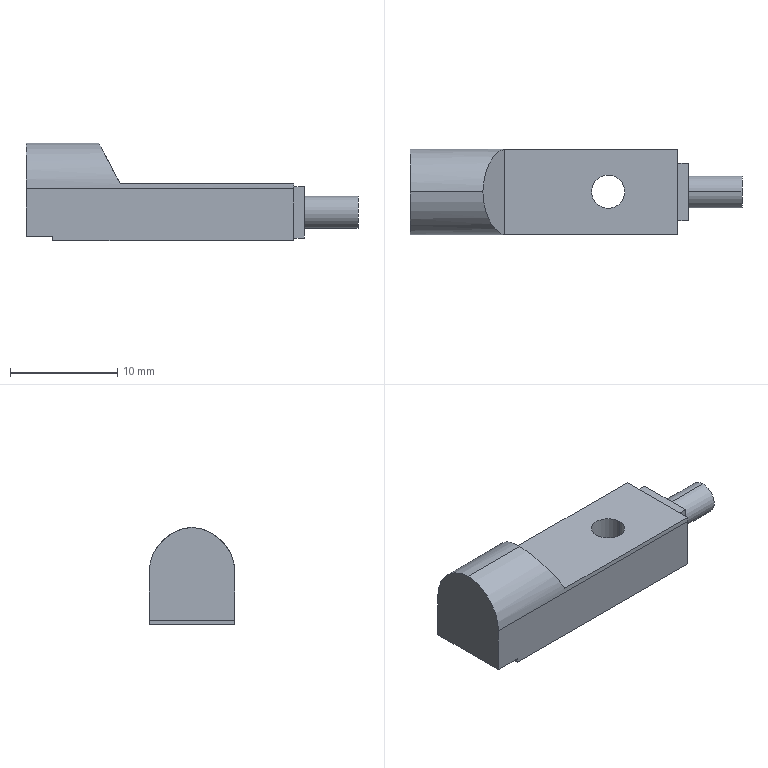Part | SolidWorks | features ICE 4, Extrusion 1, Fillet 1 | 1 solid | 21 faces | box 31 x 8 x 9.093 mm | volume 1254 mm3 | plane 15 | cylinder 6 | commonest cylinder face diameters 3 x2 3.1 x2 8.5 x2
STEP:
#1=CARTESIAN_POINT('',(31.,4.,1.15));
#2=VERTEX_POINT('',#1);
#3=CARTESIAN_POINT('',(31.,4.,4.15));
#4=VERTEX_POINT('',#3);
#5=CARTESIAN_POINT('',(31.,4.,2.65));
#6=DIRECTION('',(1.,0.,0.));
#7=DIRECTION('',(0.,0.,-1.));
#8=AXIS2_PLACEMENT_3D('',#5,#6,#7);
#9=CIRCLE('',#8,1.5);
#10=EDGE_CURVE('',#2,#4,#9,.T.);
#11=ORIENTED_EDGE('',*,*,#10,.F.);
#12=CARTESIAN_POINT('',(26.,4.,1.15));
#13=VERTEX_POINT('',#12);
#14=CARTESIAN_POINT('',(31.,4.,1.15));
#15=DIRECTION('',(-1.,0.,0.));
#16=VECTOR('',#15,1000.);
#17=LINE('',#14,#16);
#18=EDGE_CURVE('',#2,#13,#17,.T.);
#19=ORIENTED_EDGE('',*,*,#18,.T.);
#20=CARTESIAN_POINT('',(26.,4.,4.15));
#21=VERTEX_POINT('',#20);
#22=CARTESIAN_POINT('',(26.,4.,2.65));
#23=DIRECTION('',(1.,0.,0.));
#24=DIRECTION('',(0.,0.,-1.));
#25=AXIS2_PLACEMENT_3D('',#22,#23,#24);
#26=CIRCLE('',#25,1.5);
#27=EDGE_CURVE('',#13,#21,#26,.T.);
#28=ORIENTED_EDGE('',*,*,#27,.T.);
#29=CARTESIAN_POINT('',(31.,4.,4.15));
#30=DIRECTION('',(-1.,0.,0.));
#31=VECTOR('',#30,1000.);
#32=LINE('',#29,#31);
#33=EDGE_CURVE('',#4,#21,#32,.T.);
#34=ORIENTED_EDGE('',*,*,#33,.F.);
#35=EDGE_LOOP('',(#11,#19,#28,#34));
#36=FACE_OUTER_BOUND('',#35,.T.);
#37=CARTESIAN_POINT('',(31.,4.,2.65));
#38=DIRECTION('',(-1.,0.,0.));
#39=DIRECTION('',(0.,0.,1.));
#40=AXIS2_PLACEMENT_3D('',#37,#38,#39);
#41=CYLINDRICAL_SURFACE('',#40,1.5);
#42=ADVANCED_FACE('',(#36),#41,.T.);
#43=CARTESIAN_POINT('',(20.05,4.024,0.));
#44=VERTEX_POINT('',#43);
#45=CARTESIAN_POINT('',(16.95,4.024,0.));
#46=VERTEX_POINT('',#45);
#47=CARTESIAN_POINT('',(18.5,4.024,0.));
#48=DIRECTION('',(0.,0.,-1.));
#49=DIRECTION('',(-1.,0.,0.));
#50=AXIS2_PLACEMENT_3D('',#47,#48,#49);
#51=CIRCLE('',#50,1.55);
#52=EDGE_CURVE('',#44,#46,#51,.T.);
#53=ORIENTED_EDGE('',*,*,#52,.T.);
#54=CARTESIAN_POINT('',(16.95,4.024,5.3));
#55=VERTEX_POINT('',#54);
#56=CARTESIAN_POINT('',(16.95,4.024,-2.9));
#57=DIRECTION('',(0.,0.,1.));
#58=VECTOR('',#57,1000.);
#59=LINE('',#56,#58);
#60=EDGE_CURVE('',#46,#55,#59,.T.);
#61=ORIENTED_EDGE('',*,*,#60,.T.);
#62=CARTESIAN_POINT('',(20.05,4.024,5.3));
#63=VERTEX_POINT('',#62);
#64=CARTESIAN_POINT('',(18.5,4.024,5.3));
#65=DIRECTION('',(0.,0.,1.));
#66=DIRECTION('',(1.,0.,0.));
#67=AXIS2_PLACEMENT_3D('',#64,#65,#66);
#68=CIRCLE('',#67,1.55);
#69=EDGE_CURVE('',#55,#63,#68,.T.);
#70=ORIENTED_EDGE('',*,*,#69,.T.);
#71=CARTESIAN_POINT('',(20.05,4.024,-2.9));
#72=DIRECTION('',(0.,0.,1.));
#73=VECTOR('',#72,1000.);
#74=LINE('',#71,#73);
#75=EDGE_CURVE('',#44,#63,#74,.T.);
#76=ORIENTED_EDGE('',*,*,#75,.F.);
#77=EDGE_LOOP('',(#53,#61,#70,#76));
#78=FACE_OUTER_BOUND('',#77,.T.);
#79=CARTESIAN_POINT('',(18.5,4.024,-2.9));
#80=DIRECTION('',(0.,0.,1.));
#81=DIRECTION('',(1.,0.,0.));
#82=AXIS2_PLACEMENT_3D('',#79,#80,#81);
#83=CYLINDRICAL_SURFACE('',#82,1.55);
#84=ADVANCED_FACE('',(#78),#83,.F.);
#85=CARTESIAN_POINT('',(26.,1.3,0.25));
#86=VERTEX_POINT('',#85);
#87=CARTESIAN_POINT('',(26.,6.7,0.25));
#88=VERTEX_POINT('',#87);
#89=CARTESIAN_POINT('',(26.,6.7,0.25));
#90=DIRECTION('',(0.,1.,0.));
#91=VECTOR('',#90,1000.);
#92=LINE('',#89,#91);
#93=EDGE_CURVE('',#86,#88,#92,.T.);
#94=ORIENTED_EDGE('',*,*,#93,.T.);
#95=CARTESIAN_POINT('',(26.,6.7,5.05));
#96=VERTEX_POINT('',#95);
#97=CARTESIAN_POINT('',(26.,6.7,5.05));
#98=DIRECTION('',(0.,0.,1.));
#99=VECTOR('',#98,1000.);
#100=LINE('',#97,#99);
#101=EDGE_CURVE('',#88,#96,#100,.T.);
#102=ORIENTED_EDGE('',*,*,#101,.T.);
#103=CARTESIAN_POINT('',(26.,1.3,5.05));
#104=VERTEX_POINT('',#103);
#105=CARTESIAN_POINT('',(26.,6.7,5.05));
#106=DIRECTION('',(0.,-1.,0.));
#107=VECTOR('',#106,1000.);
#108=LINE('',#105,#107);
#109=EDGE_CURVE('',#96,#104,#108,.T.);
#110=ORIENTED_EDGE('',*,*,#109,.T.);
#111=CARTESIAN_POINT('',(26.,1.3,5.05));
#112=DIRECTION('',(0.,0.,-1.));
#113=VECTOR('',#112,1000.);
#114=LINE('',#111,#113);
#115=EDGE_CURVE('',#104,#86,#114,.T.);
#116=ORIENTED_EDGE('',*,*,#115,.T.);
#117=EDGE_LOOP('',(#94,#102,#110,#116));
#118=FACE_OUTER_BOUND('',#117,.T.);
#119=CARTESIAN_POINT('',(26.,4.,2.65));
#120=DIRECTION('',(1.,0.,0.));
#121=DIRECTION('',(0.,0.,-1.));
#122=AXIS2_PLACEMENT_3D('',#119,#120,#121);
#123=CIRCLE('',#122,1.5);
#124=EDGE_CURVE('',#21,#13,#123,.T.);
#125=ORIENTED_EDGE('',*,*,#124,.F.);
#126=ORIENTED_EDGE('',*,*,#27,.F.);
#127=EDGE_LOOP('',(#125,#126));
#128=FACE_BOUND('',#127,.T.);
#129=CARTESIAN_POINT('',(26.,1.3,0.25));
#130=DIRECTION('',(1.,0.,0.));
#131=DIRECTION('',(0.,0.,-1.));
#132=AXIS2_PLACEMENT_3D('',#129,#130,#131);
#133=PLANE('',#132);
#134=ADVANCED_FACE('',(#118,#128),#133,.T.);
#135=CARTESIAN_POINT('',(25.,8.,4.85));
#136=VERTEX_POINT('',#135);
#137=CARTESIAN_POINT('',(25.,8.,0.));
#138=VERTEX_POINT('',#137);
#139=CARTESIAN_POINT('',(25.,8.,9.1));
#140=DIRECTION('',(0.,0.,-1.));
#141=VECTOR('',#140,1000.);
#142=LINE('',#139,#141);
#143=EDGE_CURVE('',#136,#138,#142,.T.);
#144=ORIENTED_EDGE('',*,*,#143,.F.);
#145=CARTESIAN_POINT('',(25.,7.976,5.3));
#146=VERTEX_POINT('',#145);
#147=CARTESIAN_POINT('',(25.,3.75,4.85));
#148=DIRECTION('',(1.,0.,0.));
#149=DIRECTION('',(0.,0.,1.));
#150=AXIS2_PLACEMENT_3D('',#147,#148,#149);
#151=CIRCLE('',#150,4.25);
#152=EDGE_CURVE('',#136,#146,#151,.T.);
#153=ORIENTED_EDGE('',*,*,#152,.T.);
#154=CARTESIAN_POINT('',(25.,0.02389,5.3));
#155=VERTEX_POINT('',#154);
#156=CARTESIAN_POINT('',(25.,8.2,5.3));
#157=DIRECTION('',(0.,-1.,0.));
#158=VECTOR('',#157,1000.);
#159=LINE('',#156,#158);
#160=EDGE_CURVE('',#146,#155,#159,.T.);
#161=ORIENTED_EDGE('',*,*,#160,.T.);
#162=CARTESIAN_POINT('',(25.,0.,4.85));
#163=VERTEX_POINT('',#162);
#164=CARTESIAN_POINT('',(25.,4.25,4.85));
#165=DIRECTION('',(1.,0.,0.));
#166=DIRECTION('',(0.,0.,1.));
#167=AXIS2_PLACEMENT_3D('',#164,#165,#166);
#168=CIRCLE('',#167,4.25);
#169=EDGE_CURVE('',#155,#163,#168,.T.);
#170=ORIENTED_EDGE('',*,*,#169,.T.);
#171=CARTESIAN_POINT('',(25.,0.,0.));
#172=VERTEX_POINT('',#171);
#173=CARTESIAN_POINT('',(25.,0.,9.1));
#174=DIRECTION('',(0.,0.,-1.));
#175=VECTOR('',#174,1000.);
#176=LINE('',#173,#175);
#177=EDGE_CURVE('',#163,#172,#176,.T.);
#178=ORIENTED_EDGE('',*,*,#177,.T.);
#179=CARTESIAN_POINT('',(25.,0.,0.));
#180=DIRECTION('',(0.,1.,0.));
#181=VECTOR('',#180,1000.);
#182=LINE('',#179,#181);
#183=EDGE_CURVE('',#172,#138,#182,.T.);
#184=ORIENTED_EDGE('',*,*,#183,.T.);
#185=EDGE_LOOP('',(#144,#153,#161,#170,#178,#184));
#186=FACE_OUTER_BOUND('',#185,.T.);
#187=CARTESIAN_POINT('',(25.,1.3,0.25));
#188=VERTEX_POINT('',#187);
#189=CARTESIAN_POINT('',(25.,6.7,0.25));
#190=VERTEX_POINT('',#189);
#191=CARTESIAN_POINT('',(25.,6.7,0.25));
#192=DIRECTION('',(0.,1.,0.));
#193=VECTOR('',#192,1000.);
#194=LINE('',#191,#193);
#195=EDGE_CURVE('',#188,#190,#194,.T.);
#196=ORIENTED_EDGE('',*,*,#195,.F.);
#197=CARTESIAN_POINT('',(25.,1.3,5.05));
#198=VERTEX_POINT('',#197);
#199=CARTESIAN_POINT('',(25.,1.3,5.05));
#200=DIRECTION('',(0.,0.,-1.));
#201=VECTOR('',#200,1000.);
#202=LINE('',#199,#201);
#203=EDGE_CURVE('',#198,#188,#202,.T.);
#204=ORIENTED_EDGE('',*,*,#203,.F.);
#205=CARTESIAN_POINT('',(25.,6.7,5.05));
#206=VERTEX_POINT('',#205);
#207=CARTESIAN_POINT('',(25.,6.7,5.05));
#208=DIRECTION('',(0.,-1.,0.));
#209=VECTOR('',#208,1000.);
#210=LINE('',#207,#209);
#211=EDGE_CURVE('',#206,#198,#210,.T.);
#212=ORIENTED_EDGE('',*,*,#211,.F.);
#213=CARTESIAN_POINT('',(25.,6.7,5.05));
#214=DIRECTION('',(0.,0.,1.));
#215=VECTOR('',#214,1000.);
#216=LINE('',#213,#215);
#217=EDGE_CURVE('',#190,#206,#216,.T.);
#218=ORIENTED_EDGE('',*,*,#217,.F.);
#219=EDGE_LOOP('',(#196,#204,#212,#218));
#220=FACE_BOUND('',#219,.T.);
#221=CARTESIAN_POINT('',(25.,0.,9.1));
#222=DIRECTION('',(-1.,0.,0.));
#223=DIRECTION('',(0.,0.,1.));
#224=AXIS2_PLACEMENT_3D('',#221,#222,#223);
#225=PLANE('',#224);
#226=ADVANCED_FACE('',(#186,#220),#225,.F.);
#227=CARTESIAN_POINT('',(0.,0.,4.85));
#228=VERTEX_POINT('',#227);
#229=CARTESIAN_POINT('',(0.,4.,9.093));
#230=VERTEX_POINT('',#229);
#231=CARTESIAN_POINT('',(0.,4.25,4.85));
#232=DIRECTION('',(-1.,0.,0.));
#233=DIRECTION('',(0.,0.,-1.));
#234=AXIS2_PLACEMENT_3D('',#231,#232,#233);
#235=CIRCLE('',#234,4.25);
#236=EDGE_CURVE('',#228,#230,#235,.T.);
#237=ORIENTED_EDGE('',*,*,#236,.T.);
#238=CARTESIAN_POINT('',(0.,8.,4.85));
#239=VERTEX_POINT('',#238);
#240=CARTESIAN_POINT('',(0.,3.75,4.85));
#241=DIRECTION('',(-1.,0.,0.));
#242=DIRECTION('',(0.,0.,-1.));
#243=AXIS2_PLACEMENT_3D('',#240,#241,#242);
#244=CIRCLE('',#243,4.25);
#245=EDGE_CURVE('',#230,#239,#244,.T.);
#246=ORIENTED_EDGE('',*,*,#245,.T.);
#247=CARTESIAN_POINT('',(0.,8.,0.4));
#248=VERTEX_POINT('',#247);
#249=CARTESIAN_POINT('',(0.,8.,9.1));
#250=DIRECTION('',(0.,0.,-1.));
#251=VECTOR('',#250,1000.);
#252=LINE('',#249,#251);
#253=EDGE_CURVE('',#239,#248,#252,.T.);
#254=ORIENTED_EDGE('',*,*,#253,.T.);
#255=CARTESIAN_POINT('',(0.,0.,0.4));
#256=VERTEX_POINT('',#255);
#257=CARTESIAN_POINT('',(0.,8.2,0.4));
#258=DIRECTION('',(0.,-1.,0.));
#259=VECTOR('',#258,1000.);
#260=LINE('',#257,#259);
#261=EDGE_CURVE('',#248,#256,#260,.T.);
#262=ORIENTED_EDGE('',*,*,#261,.T.);
#263=CARTESIAN_POINT('',(0.,0.,9.1));
#264=DIRECTION('',(0.,0.,-1.));
#265=VECTOR('',#264,1000.);
#266=LINE('',#263,#265);
#267=EDGE_CURVE('',#228,#256,#266,.T.);
#268=ORIENTED_EDGE('',*,*,#267,.F.);
#269=EDGE_LOOP('',(#237,#246,#254,#262,#268));
#270=FACE_OUTER_BOUND('',#269,.T.);
#271=CARTESIAN_POINT('',(0.,0.,9.1));
#272=DIRECTION('',(1.,0.,0.));
#273=DIRECTION('',(0.,0.,-1.));
#274=AXIS2_PLACEMENT_3D('',#271,#272,#273);
#275=PLANE('',#274);
#276=ADVANCED_FACE('',(#270),#275,.F.);
#277=ORIENTED_EDGE('',*,*,#177,.F.);
#278=CARTESIAN_POINT('',(0.,0.,4.85));
#279=DIRECTION('',(-1.,0.,0.));
#280=VECTOR('',#279,1000.);
#281=LINE('',#278,#280);
#282=EDGE_CURVE('',#163,#228,#281,.T.);
#283=ORIENTED_EDGE('',*,*,#282,.T.);
#284=ORIENTED_EDGE('',*,*,#267,.T.);
#285=CARTESIAN_POINT('',(2.5,0.,0.4));
#286=VERTEX_POINT('',#285);
#287=CARTESIAN_POINT('',(0.,0.,0.4));
#288=DIRECTION('',(-1.,0.,0.));
#289=VECTOR('',#288,1000.);
#290=LINE('',#287,#289);
#291=EDGE_CURVE('',#286,#256,#290,.T.);
#292=ORIENTED_EDGE('',*,*,#291,.F.);
#293=CARTESIAN_POINT('',(2.5,0.,0.));
#294=VERTEX_POINT('',#293);
#295=CARTESIAN_POINT('',(2.5,0.,0.));
#296=DIRECTION('',(0.,0.,1.));
#297=VECTOR('',#296,1000.);
#298=LINE('',#295,#297);
#299=EDGE_CURVE('',#294,#286,#298,.T.);
#300=ORIENTED_EDGE('',*,*,#299,.F.);
#301=CARTESIAN_POINT('',(0.,0.,0.));
#302=DIRECTION('',(1.,0.,0.));
#303=VECTOR('',#302,1000.);
#304=LINE('',#301,#303);
#305=EDGE_CURVE('',#294,#172,#304,.T.);
#306=ORIENTED_EDGE('',*,*,#305,.T.);
#307=EDGE_LOOP('',(#277,#283,#284,#292,#300,#306));
#308=FACE_OUTER_BOUND('',#307,.T.);
#309=CARTESIAN_POINT('',(0.,0.,9.1));
#310=DIRECTION('',(0.,1.,0.));
#311=DIRECTION('',(0.,0.,1.));
#312=AXIS2_PLACEMENT_3D('',#309,#310,#311);
#313=PLANE('',#312);
#314=ADVANCED_FACE('',(#308),#313,.F.);
#315=ORIENTED_EDGE('',*,*,#253,.F.);
#316=CARTESIAN_POINT('',(0.,8.,4.85));
#317=DIRECTION('',(1.,0.,0.));
#318=VECTOR('',#317,1000.);
#319=LINE('',#316,#318);
#320=EDGE_CURVE('',#239,#136,#319,.T.);
#321=ORIENTED_EDGE('',*,*,#320,.T.);
#322=ORIENTED_EDGE('',*,*,#143,.T.);
#323=CARTESIAN_POINT('',(2.5,8.,0.));
#324=VERTEX_POINT('',#323);
#325=CARTESIAN_POINT('',(0.,8.,0.));
#326=DIRECTION('',(-1.,0.,0.));
#327=VECTOR('',#326,1000.);
#328=LINE('',#325,#327);
#329=EDGE_CURVE('',#138,#324,#328,.T.);
#330=ORIENTED_EDGE('',*,*,#329,.T.);
#331=CARTESIAN_POINT('',(2.5,8.,0.4));
#332=VERTEX_POINT('',#331);
#333=CARTESIAN_POINT('',(2.5,8.,9.1));
#334=DIRECTION('',(0.,0.,1.));
#335=VECTOR('',#334,1000.);
#336=LINE('',#333,#335);
#337=EDGE_CURVE('',#324,#332,#336,.T.);
#338=ORIENTED_EDGE('',*,*,#337,.T.);
#339=CARTESIAN_POINT('',(0.,8.,0.4));
#340=DIRECTION('',(-1.,0.,0.));
#341=VECTOR('',#340,1000.);
#342=LINE('',#339,#341);
#343=EDGE_CURVE('',#332,#248,#342,.T.);
#344=ORIENTED_EDGE('',*,*,#343,.T.);
#345=EDGE_LOOP('',(#315,#321,#322,#330,#338,#344));
#346=FACE_OUTER_BOUND('',#345,.T.);
#347=CARTESIAN_POINT('',(0.,8.,9.1));
#348=DIRECTION('',(0.,-1.,0.));
#349=DIRECTION('',(0.,0.,-1.));
#350=AXIS2_PLACEMENT_3D('',#347,#348,#349);
#351=PLANE('',#350);
#352=ADVANCED_FACE('',(#346),#351,.F.);
#353=ORIENTED_EDGE('',*,*,#52,.F.);
#354=CARTESIAN_POINT('',(18.5,4.024,0.));
#355=DIRECTION('',(0.,0.,-1.));
#356=DIRECTION('',(-1.,0.,0.));
#357=AXIS2_PLACEMENT_3D('',#354,#355,#356);
#358=CIRCLE('',#357,1.55);
#359=EDGE_CURVE('',#46,#44,#358,.T.);
#360=ORIENTED_EDGE('',*,*,#359,.F.);
#361=EDGE_LOOP('',(#353,#360));
#362=FACE_BOUND('',#361,.T.);
#363=CARTESIAN_POINT('',(2.5,8.,0.));
#364=DIRECTION('',(0.,-1.,0.));
#365=VECTOR('',#364,1000.);
#366=LINE('',#363,#365);
#367=EDGE_CURVE('',#324,#294,#366,.T.);
#368=ORIENTED_EDGE('',*,*,#367,.F.);
#369=ORIENTED_EDGE('',*,*,#329,.F.);
#370=ORIENTED_EDGE('',*,*,#183,.F.);
#371=ORIENTED_EDGE('',*,*,#305,.F.);
#372=EDGE_LOOP('',(#368,#369,#370,#371));
#373=FACE_OUTER_BOUND('',#372,.T.);
#374=CARTESIAN_POINT('',(0.,8.,0.));
#375=DIRECTION('',(0.,0.,-1.));
#376=DIRECTION('',(-1.,0.,0.));
#377=AXIS2_PLACEMENT_3D('',#374,#375,#376);
#378=PLANE('',#377);
#379=ADVANCED_FACE('',(#362,#373),#378,.T.);
#380=CARTESIAN_POINT('',(18.5,4.024,5.3));
#381=DIRECTION('',(0.,0.,1.));
#382=DIRECTION('',(1.,0.,0.));
#383=AXIS2_PLACEMENT_3D('',#380,#381,#382);
#384=CIRCLE('',#383,1.55);
#385=EDGE_CURVE('',#63,#55,#384,.T.);
#386=ORIENTED_EDGE('',*,*,#385,.F.);
#387=ORIENTED_EDGE('',*,*,#69,.F.);
#388=EDGE_LOOP('',(#386,#387));
#389=FACE_BOUND('',#388,.T.);
#390=ORIENTED_EDGE('',*,*,#160,.F.);
#391=CARTESIAN_POINT('',(8.8,7.976,5.3));
#392=VERTEX_POINT('',#391);
#393=CARTESIAN_POINT('',(25.,7.976,5.3));
#394=DIRECTION('',(-1.,0.,0.));
#395=VECTOR('',#394,1000.);
#396=LINE('',#393,#395);
#397=EDGE_CURVE('',#146,#392,#396,.T.);
#398=ORIENTED_EDGE('',*,*,#397,.T.);
#399=CARTESIAN_POINT('',(8.8,0.02389,5.3));
#400=VERTEX_POINT('',#399);
#401=CARTESIAN_POINT('',(8.8,8.2,5.3));
#402=DIRECTION('',(0.,-1.,0.));
#403=VECTOR('',#402,1000.);
#404=LINE('',#401,#403);
#405=EDGE_CURVE('',#392,#400,#404,.T.);
#406=ORIENTED_EDGE('',*,*,#405,.T.);
#407=CARTESIAN_POINT('',(8.8,0.02389,5.3));
#408=DIRECTION('',(1.,0.,0.));
#409=VECTOR('',#408,1000.);
#410=LINE('',#407,#409);
#411=EDGE_CURVE('',#400,#155,#410,.T.);
#412=ORIENTED_EDGE('',*,*,#411,.T.);
#413=EDGE_LOOP('',(#390,#398,#406,#412));
#414=FACE_OUTER_BOUND('',#413,.T.);
#415=CARTESIAN_POINT('',(8.8,8.2,5.3));
#416=DIRECTION('',(0.,0.,-1.));
#417=DIRECTION('',(-1.,0.,0.));
#418=AXIS2_PLACEMENT_3D('',#415,#416,#417);
#419=PLANE('',#418);
#420=ADVANCED_FACE('',(#389,#414),#419,.F.);
#421=ORIENTED_EDGE('',*,*,#405,.F.);
#422=CARTESIAN_POINT('',(6.804,4.,9.093));
#423=VERTEX_POINT('',#422);
#424=CARTESIAN_POINT('',(8.8,7.976,5.3));
#425=CARTESIAN_POINT('',(7.661,7.746,7.463));
#426=CARTESIAN_POINT('',(6.871,6.172,8.965));
#427=CARTESIAN_POINT('',(6.804,4.,9.093));
#428=(BOUNDED_CURVE()B_SPLINE_CURVE(3,(#424,#425,#426,#427),.UNSPECIFIED.,.F.,.F.)B_SPLINE_CURVE_WITH_KNOTS((4,4),(4.818,6.224),.UNSPECIFIED.)CURVE()GEOMETRIC_REPRESENTATION_ITEM()RATIONAL_B_SPLINE_CURVE((1.,0.842,0.842,1.))REPRESENTATION_ITEM(''));
#429=EDGE_CURVE('',#392,#423,#428,.T.);
#430=ORIENTED_EDGE('',*,*,#429,.T.);
#431=CARTESIAN_POINT('',(6.804,4.,9.093));
#432=CARTESIAN_POINT('',(6.871,1.828,8.965));
#433=CARTESIAN_POINT('',(7.661,0.2542,7.463));
#434=CARTESIAN_POINT('',(8.8,0.02389,5.3));
#435=(BOUNDED_CURVE()B_SPLINE_CURVE(3,(#431,#432,#433,#434),.UNSPECIFIED.,.F.,.F.)B_SPLINE_CURVE_WITH_KNOTS((4,4),(3.2,4.606),.UNSPECIFIED.)CURVE()GEOMETRIC_REPRESENTATION_ITEM()RATIONAL_B_SPLINE_CURVE((1.,0.842,0.842,1.))REPRESENTATION_ITEM(''));
#436=EDGE_CURVE('',#423,#400,#435,.T.);
#437=ORIENTED_EDGE('',*,*,#436,.T.);
#438=EDGE_LOOP('',(#421,#430,#437));
#439=FACE_OUTER_BOUND('',#438,.T.);
#440=CARTESIAN_POINT('',(6.8,8.2,9.1));
#441=DIRECTION('',(-0.8849,0.,-0.4657));
#442=DIRECTION('',(-0.4657,0.,0.8849));
#443=AXIS2_PLACEMENT_3D('',#440,#441,#442);
#444=PLANE('',#443);
#445=ADVANCED_FACE('',(#439),#444,.F.);
#446=CARTESIAN_POINT('',(2.5,8.2,0.4));
#447=DIRECTION('',(0.,-1.,0.));
#448=VECTOR('',#447,1000.);
#449=LINE('',#446,#448);
#450=EDGE_CURVE('',#332,#286,#449,.T.);
#451=ORIENTED_EDGE('',*,*,#450,.T.);
#452=ORIENTED_EDGE('',*,*,#291,.T.);
#453=ORIENTED_EDGE('',*,*,#261,.F.);
#454=ORIENTED_EDGE('',*,*,#343,.F.);
#455=EDGE_LOOP('',(#451,#452,#453,#454));
#456=FACE_OUTER_BOUND('',#455,.T.);
#457=CARTESIAN_POINT('',(0.,8.2,0.4));
#458=DIRECTION('',(0.,0.,1.));
#459=DIRECTION('',(1.,0.,0.));
#460=AXIS2_PLACEMENT_3D('',#457,#458,#459);
#461=PLANE('',#460);
#462=ADVANCED_FACE('',(#456),#461,.F.);
#463=ORIENTED_EDGE('',*,*,#367,.T.);
#464=ORIENTED_EDGE('',*,*,#299,.T.);
#465=ORIENTED_EDGE('',*,*,#450,.F.);
#466=ORIENTED_EDGE('',*,*,#337,.F.);
#467=EDGE_LOOP('',(#463,#464,#465,#466));
#468=FACE_OUTER_BOUND('',#467,.T.);
#469=CARTESIAN_POINT('',(2.5,8.2,0.));
#470=DIRECTION('',(1.,0.,0.));
#471=DIRECTION('',(0.,0.,-1.));
#472=AXIS2_PLACEMENT_3D('',#469,#470,#471);
#473=PLANE('',#472);
#474=ADVANCED_FACE('',(#468),#473,.F.);
#475=ORIENTED_EDGE('',*,*,#411,.F.);
#476=ORIENTED_EDGE('',*,*,#436,.F.);
#477=CARTESIAN_POINT('',(12.5,4.,9.093));
#478=DIRECTION('',(1.,0.,0.));
#479=VECTOR('',#478,1000.);
#480=LINE('',#477,#479);
#481=EDGE_CURVE('',#230,#423,#480,.T.);
#482=ORIENTED_EDGE('',*,*,#481,.F.);
#483=ORIENTED_EDGE('',*,*,#236,.F.);
#484=ORIENTED_EDGE('',*,*,#282,.F.);
#485=ORIENTED_EDGE('',*,*,#169,.F.);
#486=EDGE_LOOP('',(#475,#476,#482,#483,#484,#485));
#487=FACE_OUTER_BOUND('',#486,.T.);
#488=CARTESIAN_POINT('',(0.,4.25,4.85));
#489=DIRECTION('',(1.,0.,0.));
#490=DIRECTION('',(0.,0.,-1.));
#491=AXIS2_PLACEMENT_3D('',#488,#489,#490);
#492=CYLINDRICAL_SURFACE('',#491,4.25);
#493=ADVANCED_FACE('',(#487),#492,.T.);
#494=ORIENTED_EDGE('',*,*,#152,.F.);
#495=ORIENTED_EDGE('',*,*,#320,.F.);
#496=ORIENTED_EDGE('',*,*,#245,.F.);
#497=ORIENTED_EDGE('',*,*,#481,.T.);
#498=ORIENTED_EDGE('',*,*,#429,.F.);
#499=ORIENTED_EDGE('',*,*,#397,.F.);
#500=EDGE_LOOP('',(#494,#495,#496,#497,#498,#499));
#501=FACE_OUTER_BOUND('',#500,.T.);
#502=CARTESIAN_POINT('',(0.,3.75,4.85));
#503=DIRECTION('',(-1.,0.,0.));
#504=DIRECTION('',(0.,0.,1.));
#505=AXIS2_PLACEMENT_3D('',#502,#503,#504);
#506=CYLINDRICAL_SURFACE('',#505,4.25);
#507=ADVANCED_FACE('',(#501),#506,.T.);
#508=ORIENTED_EDGE('',*,*,#60,.F.);
#509=ORIENTED_EDGE('',*,*,#359,.T.);
#510=ORIENTED_EDGE('',*,*,#75,.T.);
#511=ORIENTED_EDGE('',*,*,#385,.T.);
#512=EDGE_LOOP('',(#508,#509,#510,#511));
#513=FACE_OUTER_BOUND('',#512,.T.);
#514=CARTESIAN_POINT('',(18.5,4.024,-2.9));
#515=DIRECTION('',(0.,0.,1.));
#516=DIRECTION('',(1.,0.,0.));
#517=AXIS2_PLACEMENT_3D('',#514,#515,#516);
#518=CYLINDRICAL_SURFACE('',#517,1.55);
#519=ADVANCED_FACE('',(#513),#518,.F.);
#520=ORIENTED_EDGE('',*,*,#195,.T.);
#521=CARTESIAN_POINT('',(26.,6.7,0.25));
#522=DIRECTION('',(-1.,0.,0.));
#523=VECTOR('',#522,1000.);
#524=LINE('',#521,#523);
#525=EDGE_CURVE('',#88,#190,#524,.T.);
#526=ORIENTED_EDGE('',*,*,#525,.F.);
#527=ORIENTED_EDGE('',*,*,#93,.F.);
#528=CARTESIAN_POINT('',(26.,1.3,0.25));
#529=DIRECTION('',(-1.,0.,0.));
#530=VECTOR('',#529,1000.);
#531=LINE('',#528,#530);
#532=EDGE_CURVE('',#86,#188,#531,.T.);
#533=ORIENTED_EDGE('',*,*,#532,.T.);
#534=EDGE_LOOP('',(#520,#526,#527,#533));
#535=FACE_OUTER_BOUND('',#534,.T.);
#536=CARTESIAN_POINT('',(26.,6.7,0.25));
#537=DIRECTION('',(0.,0.,1.));
#538=DIRECTION('',(0.,-1.,0.));
#539=AXIS2_PLACEMENT_3D('',#536,#537,#538);
#540=PLANE('',#539);
#541=ADVANCED_FACE('',(#535),#540,.F.);
#542=ORIENTED_EDGE('',*,*,#217,.T.);
#543=CARTESIAN_POINT('',(26.,6.7,5.05));
#544=DIRECTION('',(-1.,0.,0.));
#545=VECTOR('',#544,1000.);
#546=LINE('',#543,#545);
#547=EDGE_CURVE('',#96,#206,#546,.T.);
#548=ORIENTED_EDGE('',*,*,#547,.F.);
#549=ORIENTED_EDGE('',*,*,#101,.F.);
#550=ORIENTED_EDGE('',*,*,#525,.T.);
#551=EDGE_LOOP('',(#542,#548,#549,#550));
#552=FACE_OUTER_BOUND('',#551,.T.);
#553=CARTESIAN_POINT('',(26.,6.7,5.05));
#554=DIRECTION('',(0.,-1.,0.));
#555=DIRECTION('',(0.,0.,-1.));
#556=AXIS2_PLACEMENT_3D('',#553,#554,#555);
#557=PLANE('',#556);
#558=ADVANCED_FACE('',(#552),#557,.F.);
#559=ORIENTED_EDGE('',*,*,#211,.T.);
#560=CARTESIAN_POINT('',(26.,1.3,5.05));
#561=DIRECTION('',(-1.,0.,0.));
#562=VECTOR('',#561,1000.);
#563=LINE('',#560,#562);
#564=EDGE_CURVE('',#104,#198,#563,.T.);
#565=ORIENTED_EDGE('',*,*,#564,.F.);
#566=ORIENTED_EDGE('',*,*,#109,.F.);
#567=ORIENTED_EDGE('',*,*,#547,.T.);
#568=EDGE_LOOP('',(#559,#565,#566,#567));
#569=FACE_OUTER_BOUND('',#568,.T.);
#570=CARTESIAN_POINT('',(26.,6.7,5.05));
#571=DIRECTION('',(0.,0.,-1.));
#572=DIRECTION('',(0.,1.,0.));
#573=AXIS2_PLACEMENT_3D('',#570,#571,#572);
#574=PLANE('',#573);
#575=ADVANCED_FACE('',(#569),#574,.F.);
#576=ORIENTED_EDGE('',*,*,#203,.T.);
#577=ORIENTED_EDGE('',*,*,#532,.F.);
#578=ORIENTED_EDGE('',*,*,#115,.F.);
#579=ORIENTED_EDGE('',*,*,#564,.T.);
#580=EDGE_LOOP('',(#576,#577,#578,#579));
#581=FACE_OUTER_BOUND('',#580,.T.);
#582=CARTESIAN_POINT('',(26.,1.3,5.05));
#583=DIRECTION('',(0.,1.,0.));
#584=DIRECTION('',(0.,0.,1.));
#585=AXIS2_PLACEMENT_3D('',#582,#583,#584);
#586=PLANE('',#585);
#587=ADVANCED_FACE('',(#581),#586,.F.);
#588=ORIENTED_EDGE('',*,*,#18,.F.);
#589=CARTESIAN_POINT('',(31.,4.,2.65));
#590=DIRECTION('',(1.,0.,0.));
#591=DIRECTION('',(0.,0.,-1.));
#592=AXIS2_PLACEMENT_3D('',#589,#590,#591);
#593=CIRCLE('',#592,1.5);
#594=EDGE_CURVE('',#4,#2,#593,.T.);
#595=ORIENTED_EDGE('',*,*,#594,.F.);
#596=ORIENTED_EDGE('',*,*,#33,.T.);
#597=ORIENTED_EDGE('',*,*,#124,.T.);
#598=EDGE_LOOP('',(#588,#595,#596,#597));
#599=FACE_OUTER_BOUND('',#598,.T.);
#600=CARTESIAN_POINT('',(31.,4.,2.65));
#601=DIRECTION('',(-1.,0.,0.));
#602=DIRECTION('',(0.,0.,1.));
#603=AXIS2_PLACEMENT_3D('',#600,#601,#602);
#604=CYLINDRICAL_SURFACE('',#603,1.5);
#605=ADVANCED_FACE('',(#599),#604,.T.);
#606=ORIENTED_EDGE('',*,*,#594,.T.);
#607=ORIENTED_EDGE('',*,*,#10,.T.);
#608=EDGE_LOOP('',(#606,#607));
#609=FACE_OUTER_BOUND('',#608,.T.);
#610=CARTESIAN_POINT('',(31.,4.,2.65));
#611=DIRECTION('',(1.,0.,0.));
#612=DIRECTION('',(0.,0.,-1.));
#613=AXIS2_PLACEMENT_3D('',#610,#611,#612);
#614=PLANE('',#613);
#615=ADVANCED_FACE('',(#609),#614,.T.);
#616=CLOSED_SHELL('',(#42,#84,#134,#226,#276,#314,#352,#379,#420,#445,#462,#474,#493,#507,#519,#541,#558,#575,#587,#605,#615));
#617=MANIFOLD_SOLID_BREP('',#616);
#618=CARTESIAN_POINT('',(0.,0.,0.));
#619=DIRECTION('',(0.,0.,1.));
#620=DIRECTION('',(1.,0.,0.));
#621=AXIS2_PLACEMENT_3D('',#618,#619,#620);
#622=(LENGTH_UNIT()NAMED_UNIT(*)SI_UNIT(.MILLI.,.METRE.));
#623=UNCERTAINTY_MEASURE_WITH_UNIT(LENGTH_MEASURE(0.00001),#622,'','');
#624=(NAMED_UNIT(*)PLANE_ANGLE_UNIT()SI_UNIT($,.RADIAN.));
#625=(NAMED_UNIT(*)SI_UNIT($,.STERADIAN.)SOLID_ANGLE_UNIT());
#626=(GEOMETRIC_REPRESENTATION_CONTEXT(3)GLOBAL_UNCERTAINTY_ASSIGNED_CONTEXT((#623))GLOBAL_UNIT_ASSIGNED_CONTEXT((#622,#624,#625))REPRESENTATION_CONTEXT('',''));
#627=ADVANCED_BREP_SHAPE_REPRESENTATION('',(#617,#621),#626);